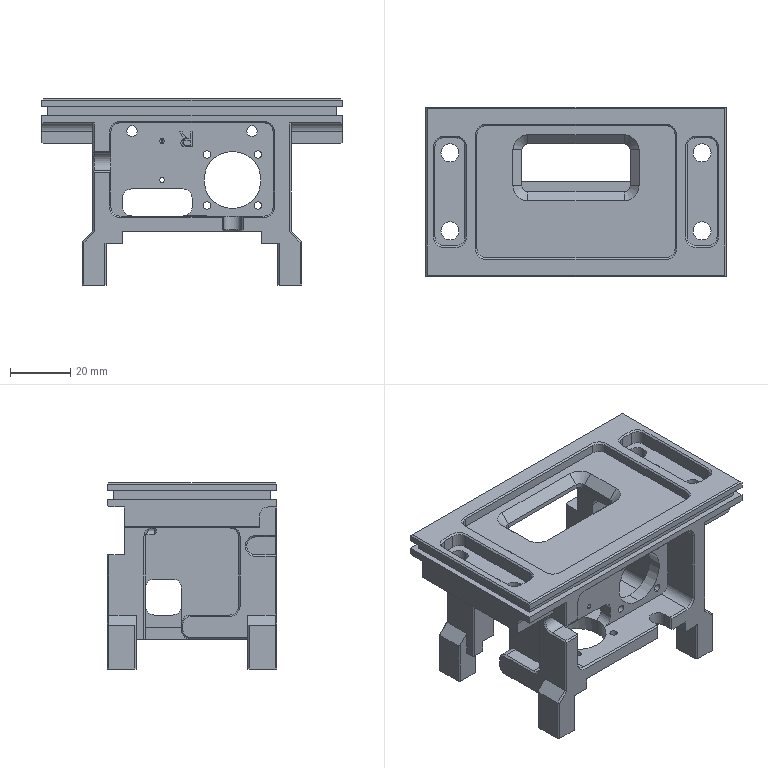Part | 1 solid | 365 faces | box 100 x 56.5 x 62 mm | volume 79263 mm3 | plane 202 | cylinder 104 | cone 53 | other 6 | commonest cylinder face diameters 6 x56 2.5 x30 4 x6 1.6 x4 3.5 x4 19 x4